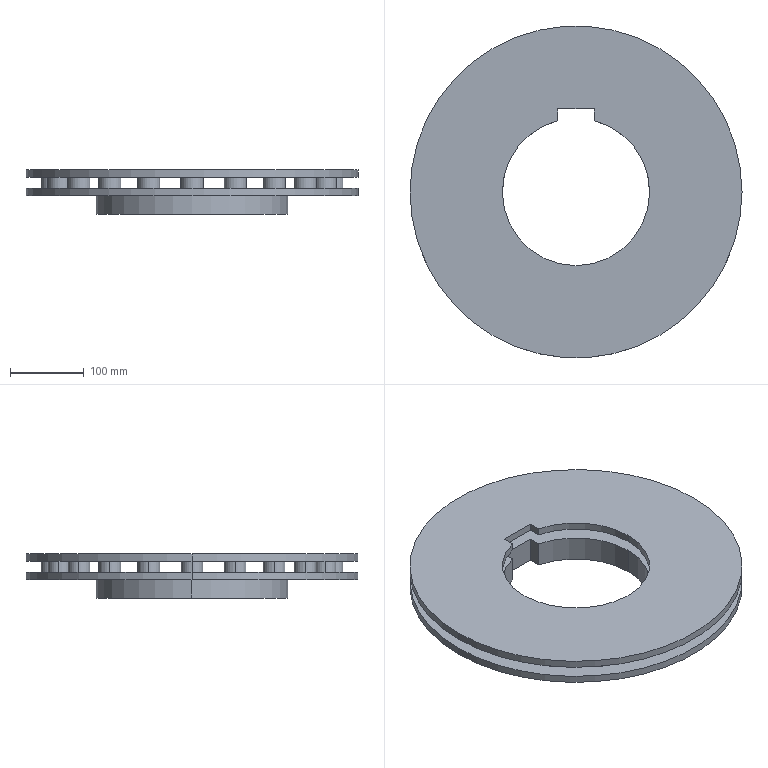Part | SolidWorks | features ICE 3, Extrusion 1, MirrorSolid 1 | 1 solid | 63 faces | box 451 x 451 x 60 mm | volume 3289063 mm3 | cylinder 52 | plane 11 | commonest cylinder face diameters 30 x40 200 x6 451 x4 260 x2